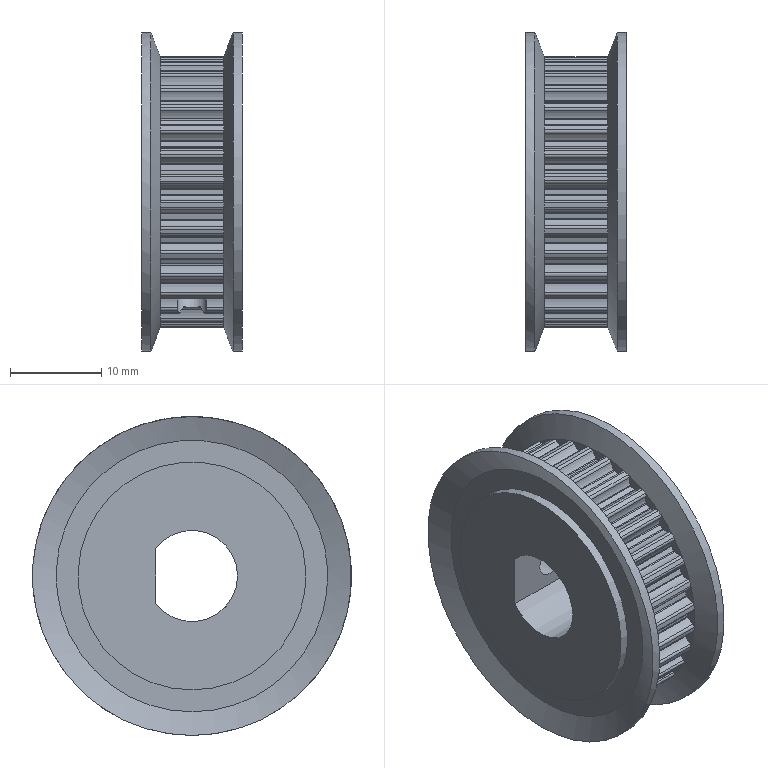Part | NX | features OFFSET_REGION 2, BREP 1 | 1 solid | 352 faces | box 11 x 35 x 35 mm | volume 6439 mm3 | cylinder 279 | plane 69 | cone 4 | commonest cylinder face diameters 0.3 x69 0.56 x68 3.95 x68 27.58 x34 29.8 x33 3.242 x2